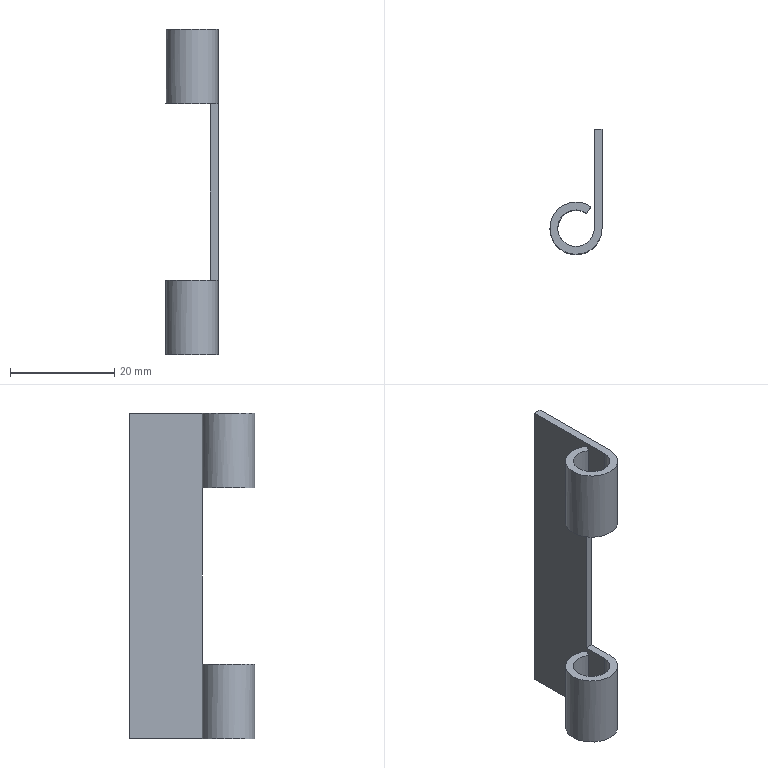Part | STEP file | RJWD-DY-0102_X2_5DE667DC95E8_30 | 1 solid | 14 faces | box 10 x 24 x 62.5 mm | volume 2502 mm3 | plane 10 | cylinder 4 | commonest cylinder face diameters 7 x2 10 x2